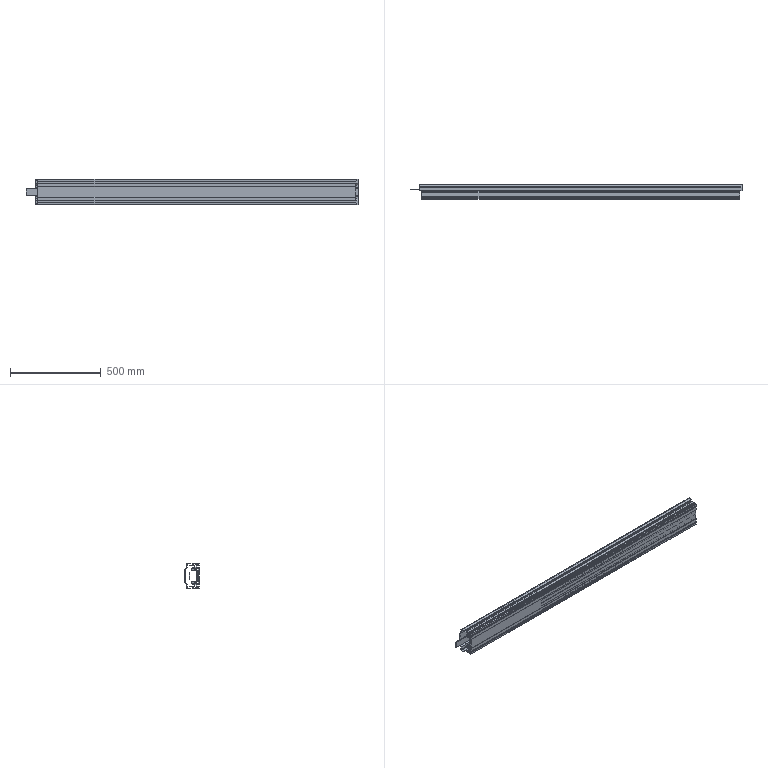Part | NX | features BREP 5 | 5 solids | 360 faces | box 1825 x 79 x 140 mm | volume 4842399 mm3 | plane 240 | cylinder 95 | cone 25 | commonest cylinder face diameters 5 x18 0.4 x16 0.6 x12 3 x12 2 x10 4.9 x9